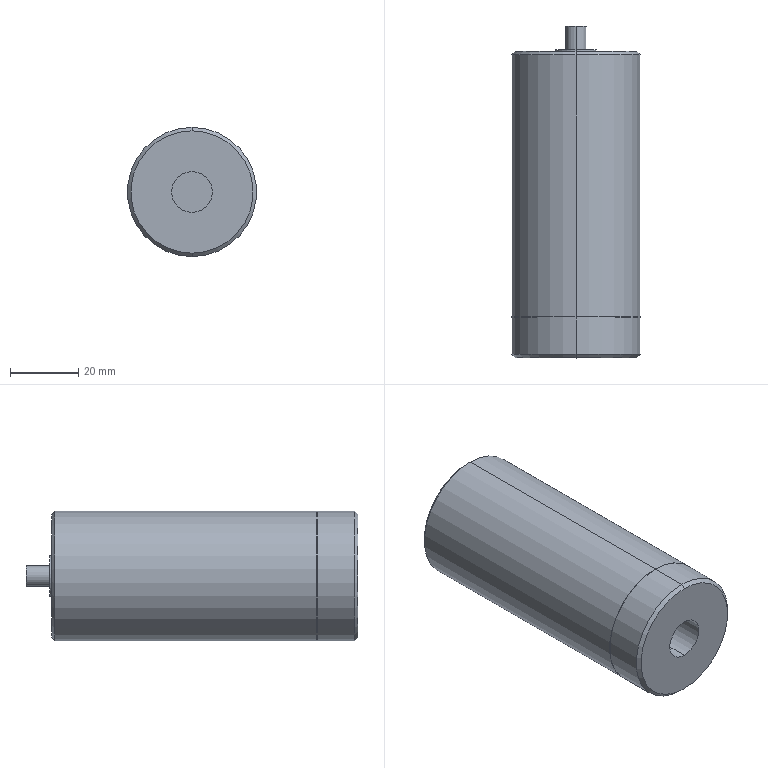Part | STEP file | PN_0007 | 22 solids | 108 faces | box 38 x 97.6 x 38 mm | volume 92613 mm3 | torus 72 | cylinder 20 | plane 12 | cone 4 | commonest cylinder face diameters 12 x6 38 x4 6 x2 12.2 x2 17.8 x2 17.98 x2